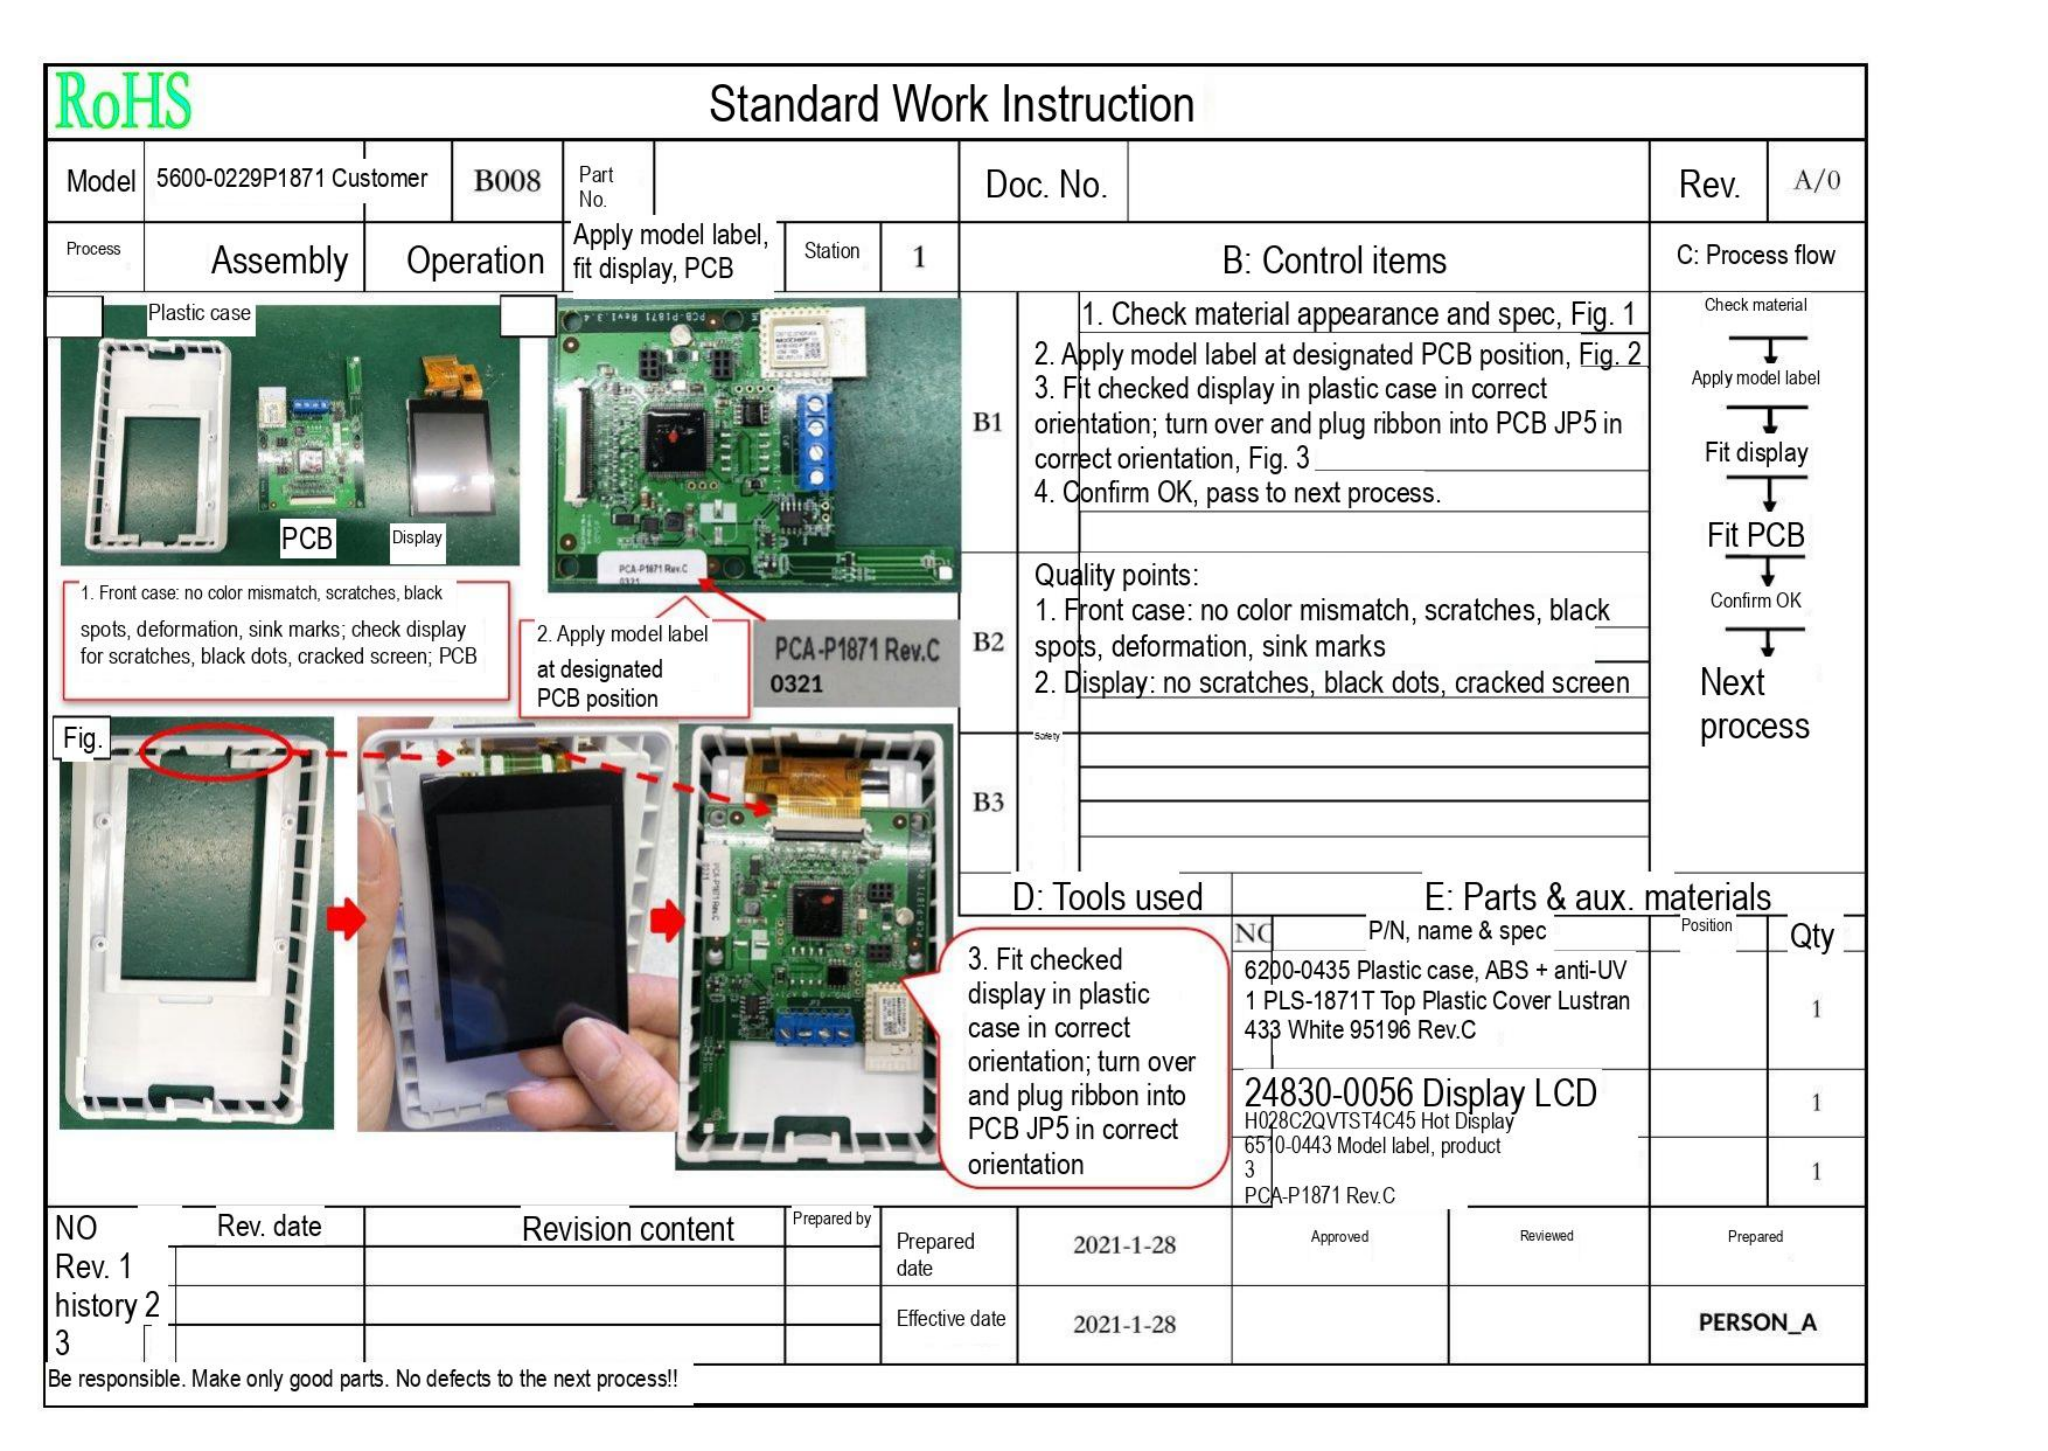RoHS

# Standard Work Instruction

| Model | 5600-0229P1871 Customer | B008 | Part No. | | Doc. No. | | Rev. | A/0 |
|---|---|---|---|---|---|---|---|---|

| Process | Assembly | Operation | Apply model label, fit display, PCB | Station | 1 | B: Control items | C: Process flow |
|---|---|---|---|---|---|---|---|

Plastic case

PCB

Display

1. Front case: no color mismatch, scratches, black spots, deformation, sink marks; check display for scratches, black dots, cracked screen; PCB

PCA-P1871 Rev.C
0321

2. Apply model label at designated PCB position

PCA-P1871 Rev.C
0321

Fig.

3. Fit checked display in plastic case in correct orientation; turn over and plug ribbon into PCB JP5 in correct orientation

| | |
|---|---|
| B1 | 1. Check material appearance and spec, Fig. 1<br>2. Apply model label at designated PCB position, Fig. 2<br>3. Fit checked display in plastic case in correct orientation; turn over and plug ribbon into PCB JP5 in correct orientation, Fig. 3<br>4. Confirm OK, pass to next process. |
| B2 | Quality points:<br>1. Front case: no color mismatch, scratches, black spots, deformation, sink marks<br>2. Display: no scratches, black dots, cracked screen |
| B3 | Safety |

C: Process flow
Check material
Apply model label
Fit display
Fit PCB
Confirm OK
Next process

D: Tools used

E: Parts & aux. materials

| NO | P/N, name & spec | Position | Qty |
|---|---|---|---|
| 1 | 6200-0435 Plastic case, ABS + anti-UV PLS-1871T Top Plastic Cover Lustran 433 White 95196 Rev.C | | 1 |
| | 24830-0056 Display LCD H028C2QVTST4C45 Hot Display | | 1 |
| 3 | 6510-0443 Model label, product PCA-P1871 Rev.C | | 1 |

| NO | Rev. date | Revision content | Prepared by |
|---|---|---|---|
| Rev. history 1 | | | |
| 2 | | | |
| 3 | | | |

| Prepared date | 2021-1-28 | Approved | Reviewed | Prepared |
|---|---|---|---|---|
| Effective date | 2021-1-28 | | | PERSON_A |

Be responsible. Make only good parts. No defects to the next process!!
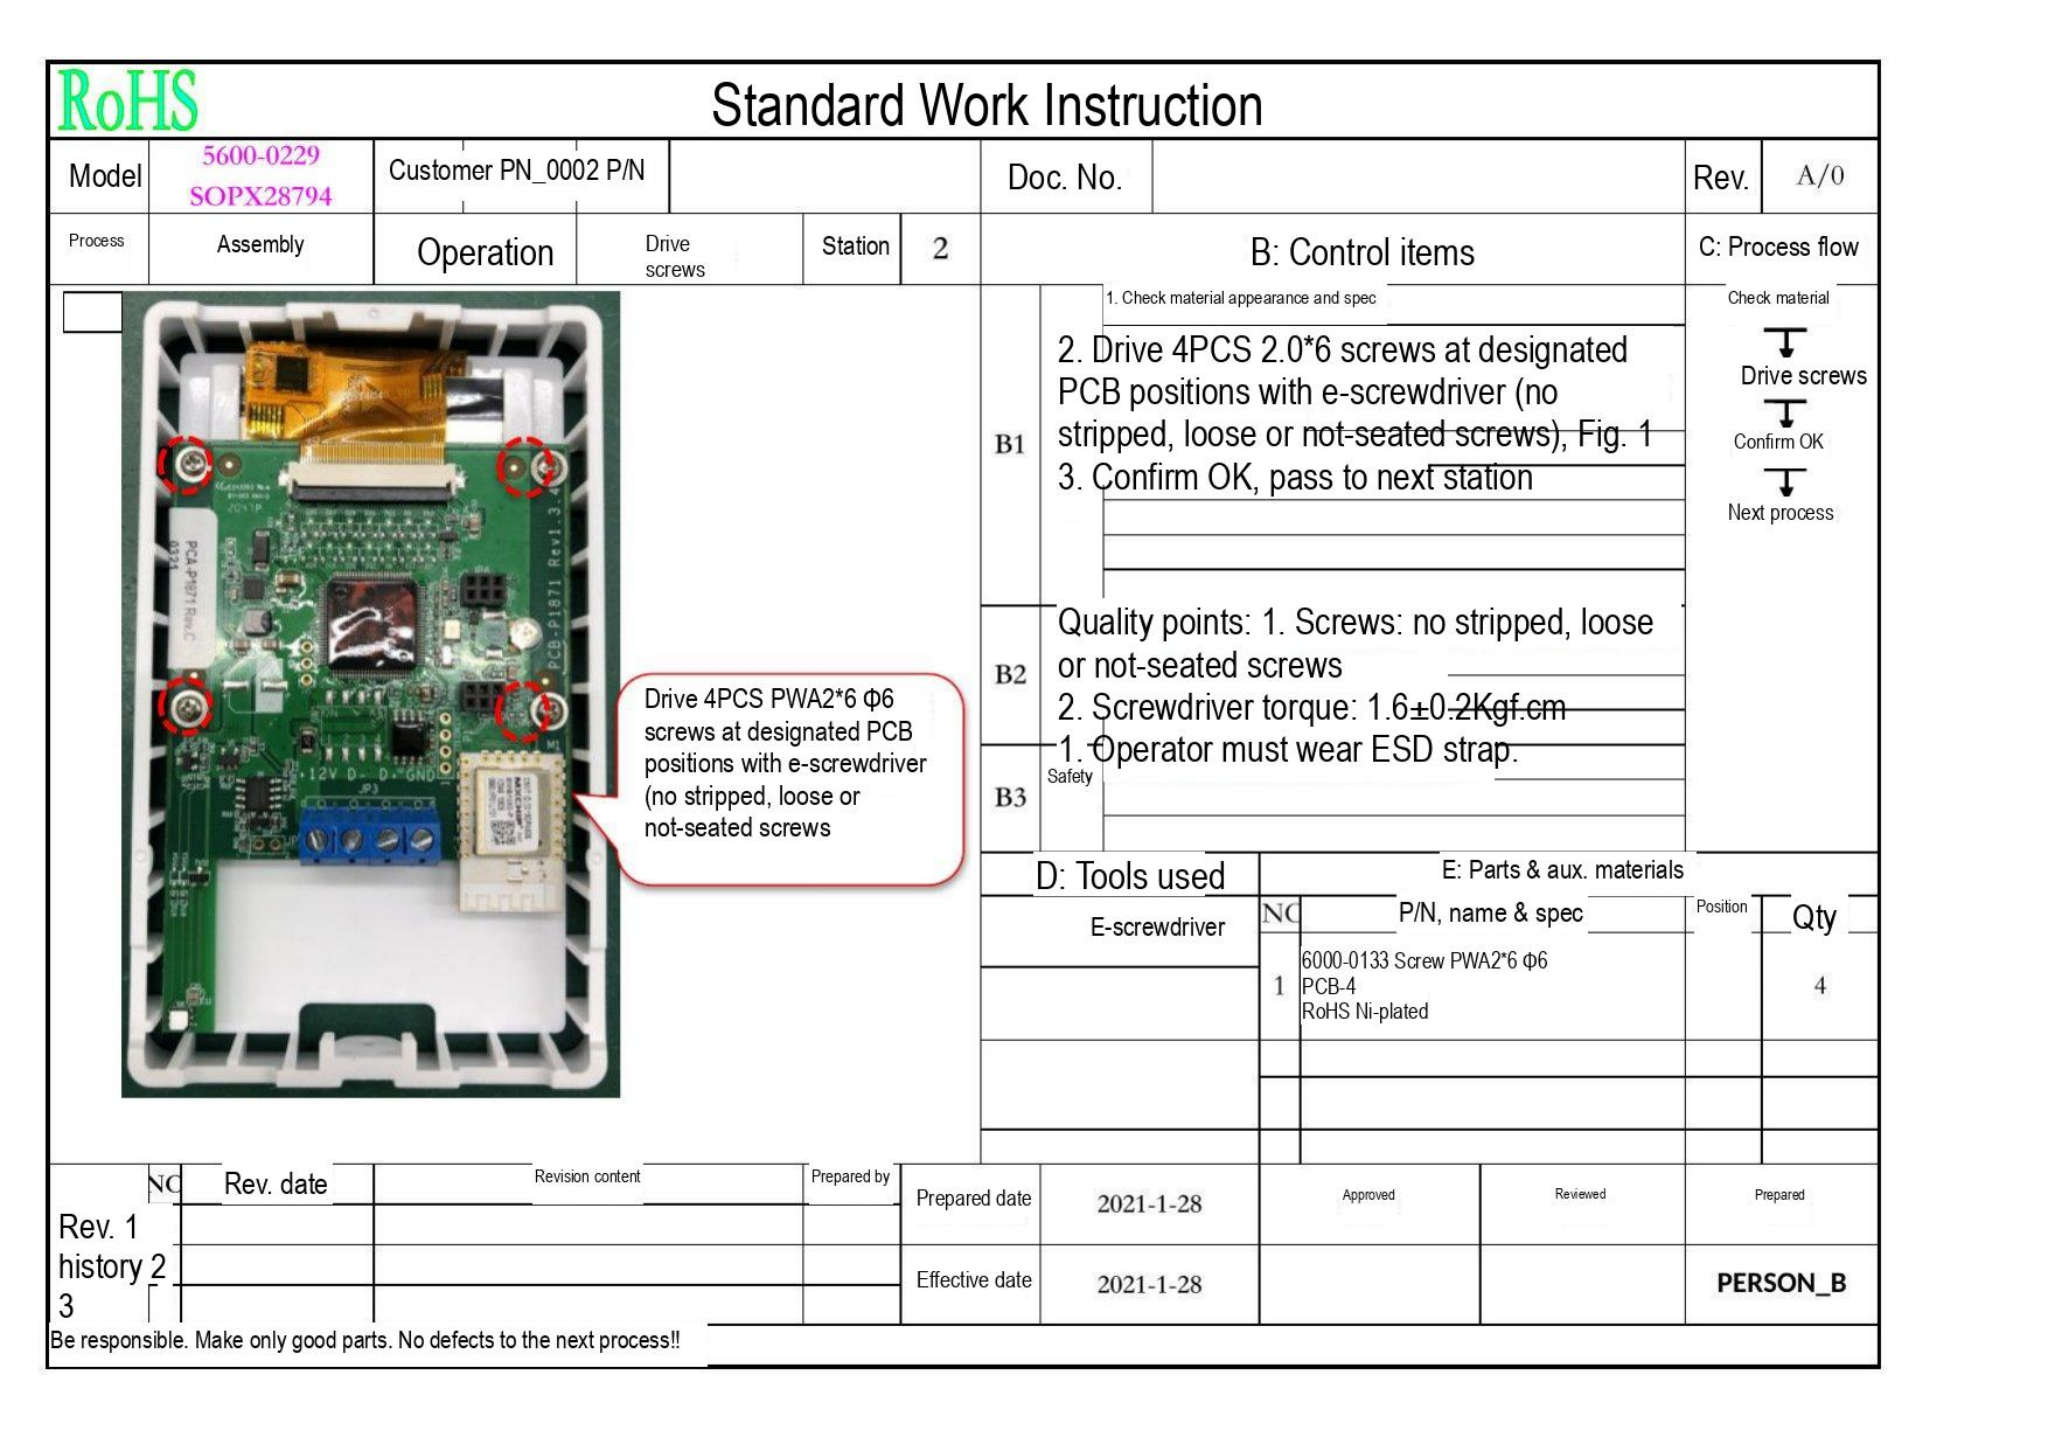RoHS

# Standard Work Instruction

| Model | 5600-0229 SOPX28794 | Customer PN_0002 P/N | | Doc. No. | | Rev. | A/0 |
|---|---|---|---|---|---|---|---|
| Process | Assembly | Operation | Drive screws | Station | 2 | | |

PCA-P1871 Rev.C

PCB-P1871 Rev1.3

12V D- D+ GND

JP3

Drive 4PCS PWA2*6 Φ6 screws at designated PCB positions with e-screwdriver (no stripped, loose or not-seated screws

**B: Control items**

| | | |
|---|---|---|
| B1 | | 1. Check material appearance and spec<br>2. Drive 4PCS 2.0*6 screws at designated PCB positions with e-screwdriver (no stripped, loose or not-seated screws), Fig. 1<br>3. Confirm OK, pass to next station |
| B2 | | Quality points: 1. Screws: no stripped, loose or not-seated screws<br>2. Screwdriver torque: 1.6±0.2Kgf.cm |
| B3 | Safety | 1. Operator must wear ESD strap. |

**C: Process flow**

Check material
↓
Drive screws
↓
Confirm OK
↓
Next process

**D: Tools used**

| D: Tools used |
|---|
| E-screwdriver |

**E: Parts & aux. materials**

| NO | P/N, name & spec | Position | Qty |
|---|---|---|---|
| 1 | 6000-0133 Screw PWA2*6 Φ6<br>PCB-4<br>RoHS Ni-plated | | 4 |

| Rev. history | NO | Rev. date | Revision content | Prepared by |
|---|---|---|---|---|
| | 1 | | | |
| | 2 | | | |
| | 3 | | | |

| Prepared date | 2021-1-28 | Approved | Reviewed | Prepared |
|---|---|---|---|---|
| Effective date | 2021-1-28 | | | PERSON_B |

Be responsible. Make only good parts. No defects to the next process!!
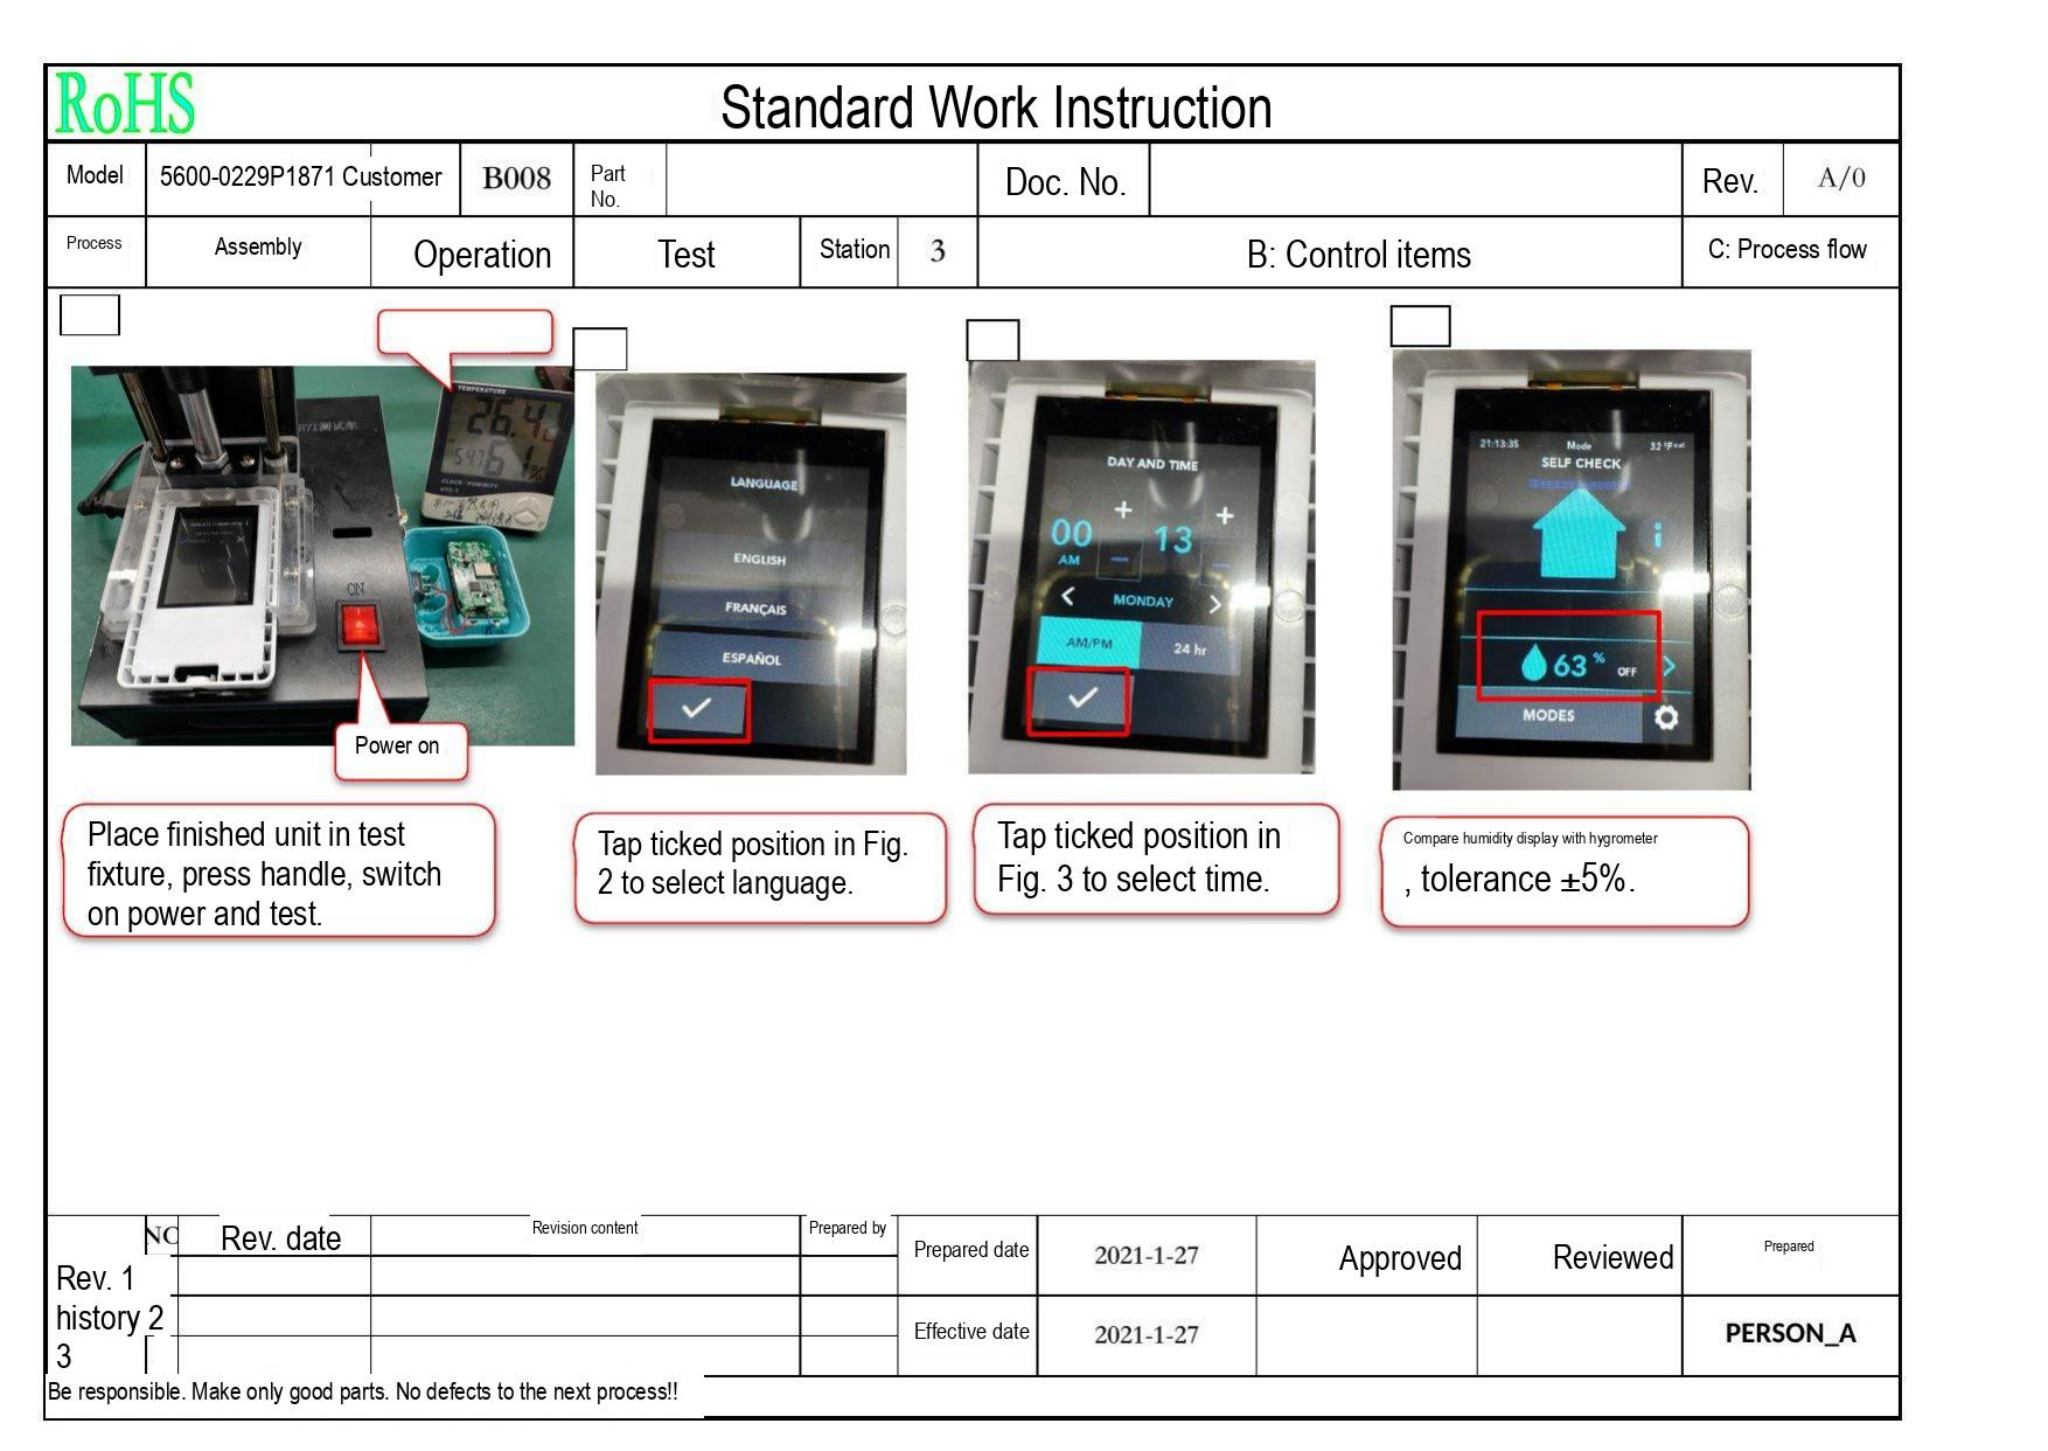RoHS

Standard Work Instruction

| Model | 5600-0229P1871 Customer | B008 | Part No. | | Doc. No. | | Rev. | A/0 |
|---|---|---|---|---|---|---|---|---|
| Process | Assembly | Operation | Test | Station | 3 | B: Control items | | C: Process flow |

TEMPERATURE
26.4
54%
61%
CLOCK HUMIDITY

ON

Power on

Place finished unit in test fixture, press handle, switch on power and test.

LANGUAGE
ENGLISH
FRANÇAIS
ESPAÑOL

Tap ticked position in Fig. 2 to select language.

DAY AND TIME
00
AM
13
MONDAY
AM/PM
24 hr

Tap ticked position in Fig. 3 to select time.

21:13:35
Mode
SELF CHECK
63 %
OFF
MODES

Compare humidity display with hygrometer
, tolerance ±5%.

| Rev. history | NO | Rev. date | Revision content | Prepared by | Prepared date | 2021-1-27 | Approved | Reviewed | Prepared |
|---|---|---|---|---|---|---|---|---|---|
| | 1 | | | | | | | | |
| | 2 | | | | Effective date | 2021-1-27 | | | PERSON_A |
| | 3 | | | | | | | | |

Be responsible. Make only good parts. No defects to the next process!!
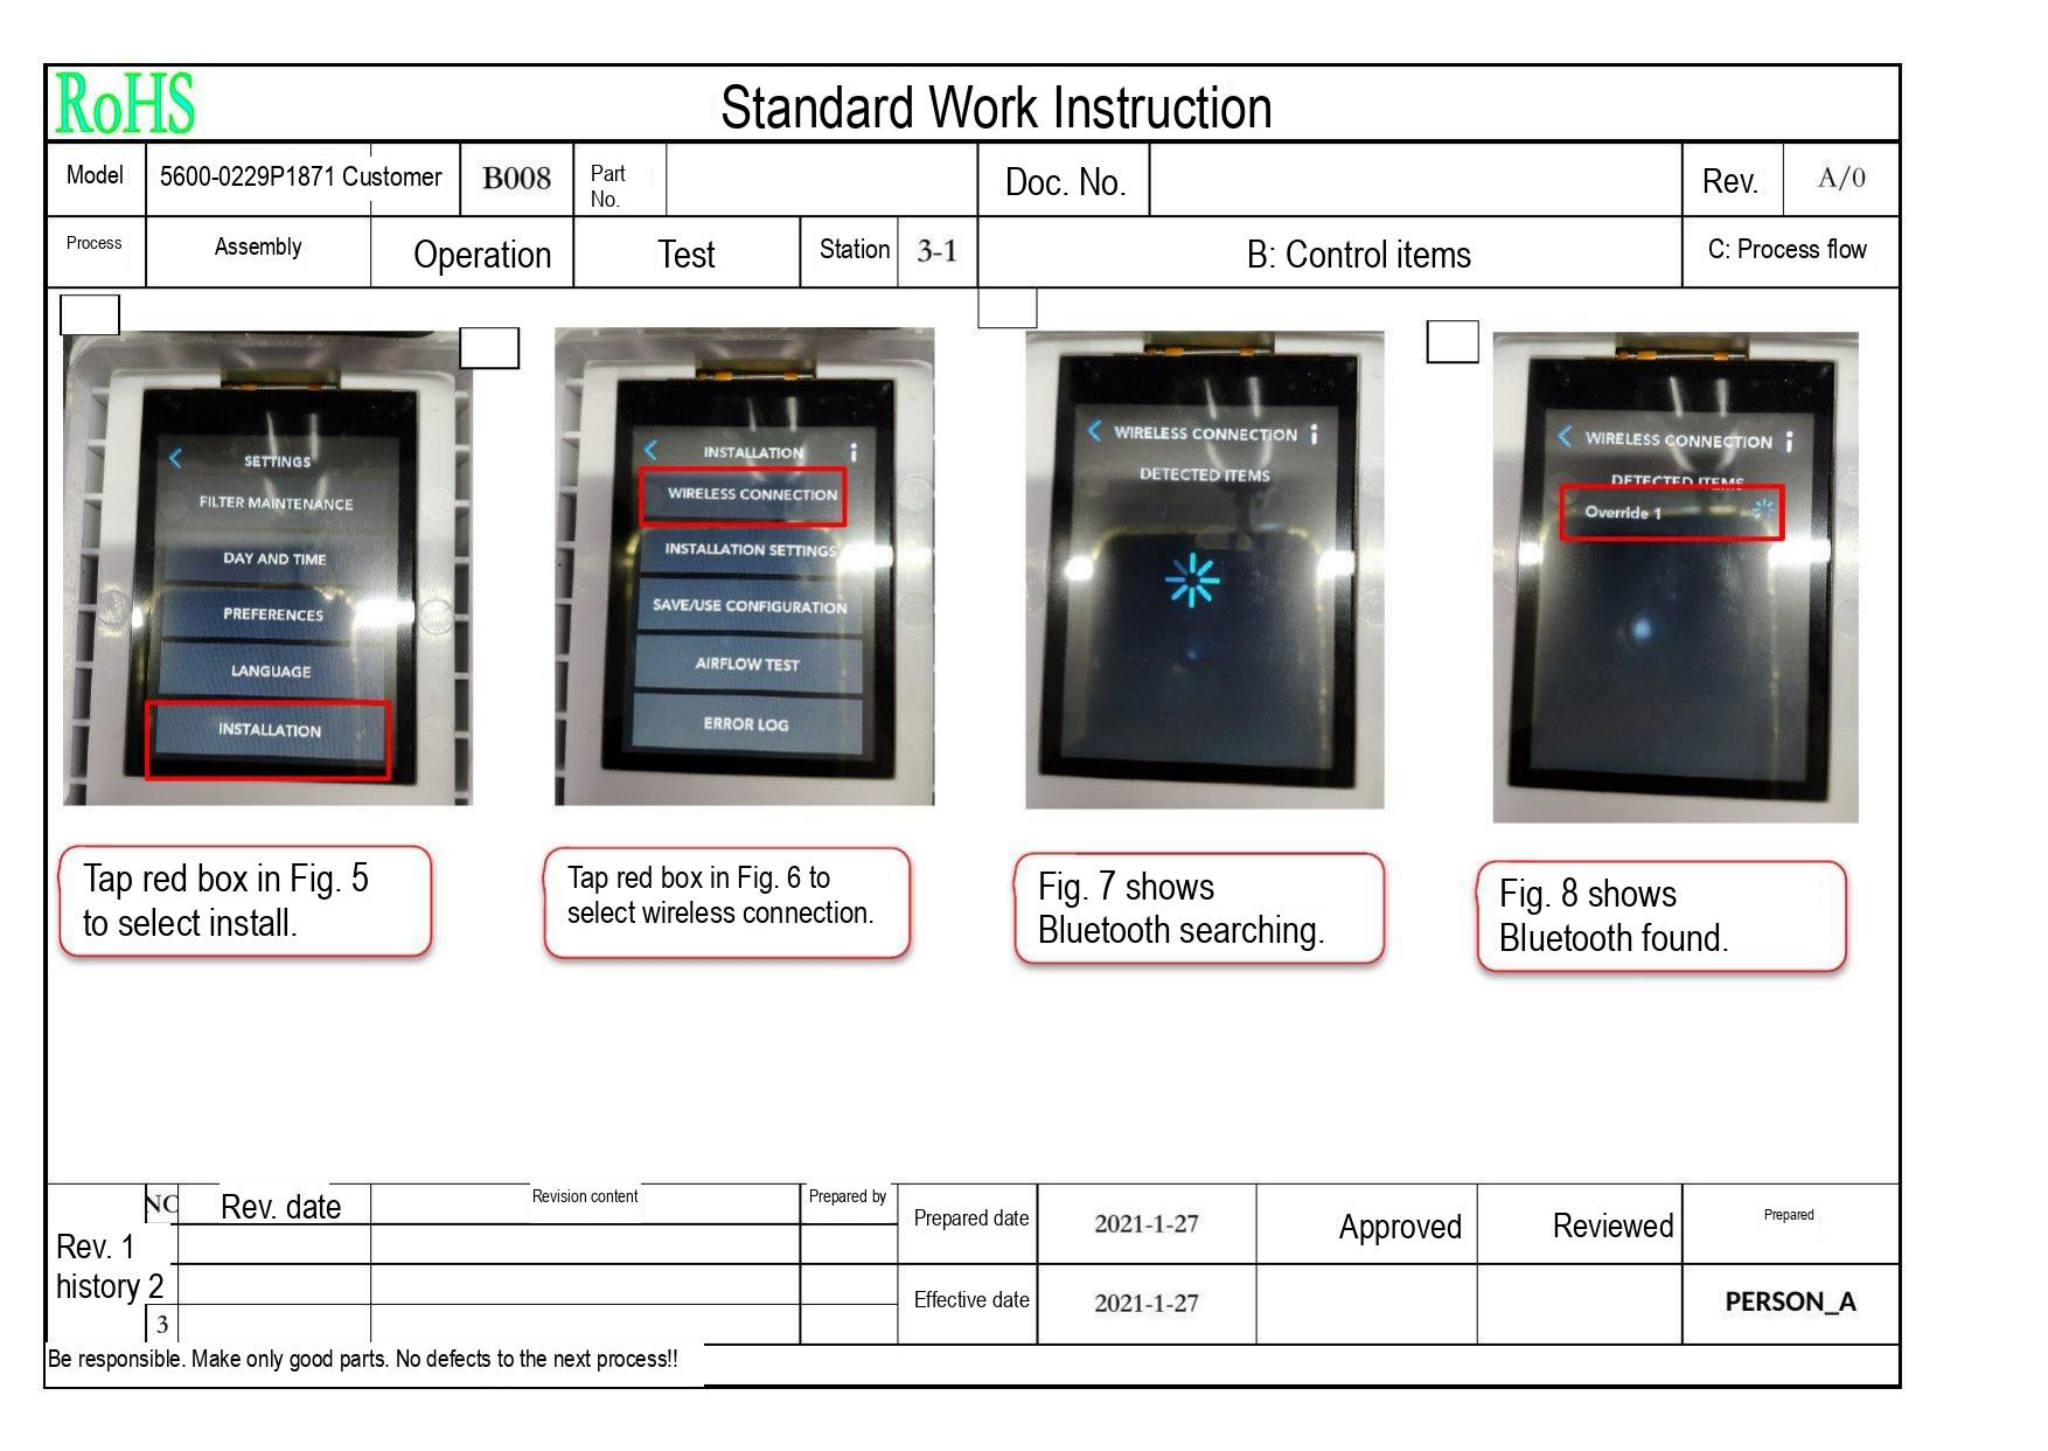RoHS

Standard Work Instruction

| Model | 5600-0229P1871 | Customer | B008 | Part No. | | Doc. No. | | Rev. | A/0 |
|---|---|---|---|---|---|---|---|---|---|
| Process | Assembly | Operation | Test | Station | 3-1 | B: Control items | | C: Process flow | |

SETTINGS
FILTER MAINTENANCE
DAY AND TIME
PREFERENCES
LANGUAGE
INSTALLATION

INSTALLATION
WIRELESS CONNECTION
INSTALLATION SETTINGS
SAVE/USE CONFIGURATION
AIRFLOW TEST
ERROR LOG

WIRELESS CONNECTION
DETECTED ITEMS

WIRELESS CONNECTION
DETECTED ITEMS
Override 1

Tap red box in Fig. 5 to select install.

Tap red box in Fig. 6 to select wireless connection.

Fig. 7 shows Bluetooth searching.

Fig. 8 shows Bluetooth found.

| Rev. history | NO | Rev. date | Revision content | Prepared by | Prepared date | 2021-1-27 | Approved | Reviewed | Prepared |
|---|---|---|---|---|---|---|---|---|---|
| | 1 | | | | | | | | |
| | 2 | | | | Effective date | 2021-1-27 | | | PERSON_A |
| | 3 | | | | | | | | |

Be responsible. Make only good parts. No defects to the next process!!
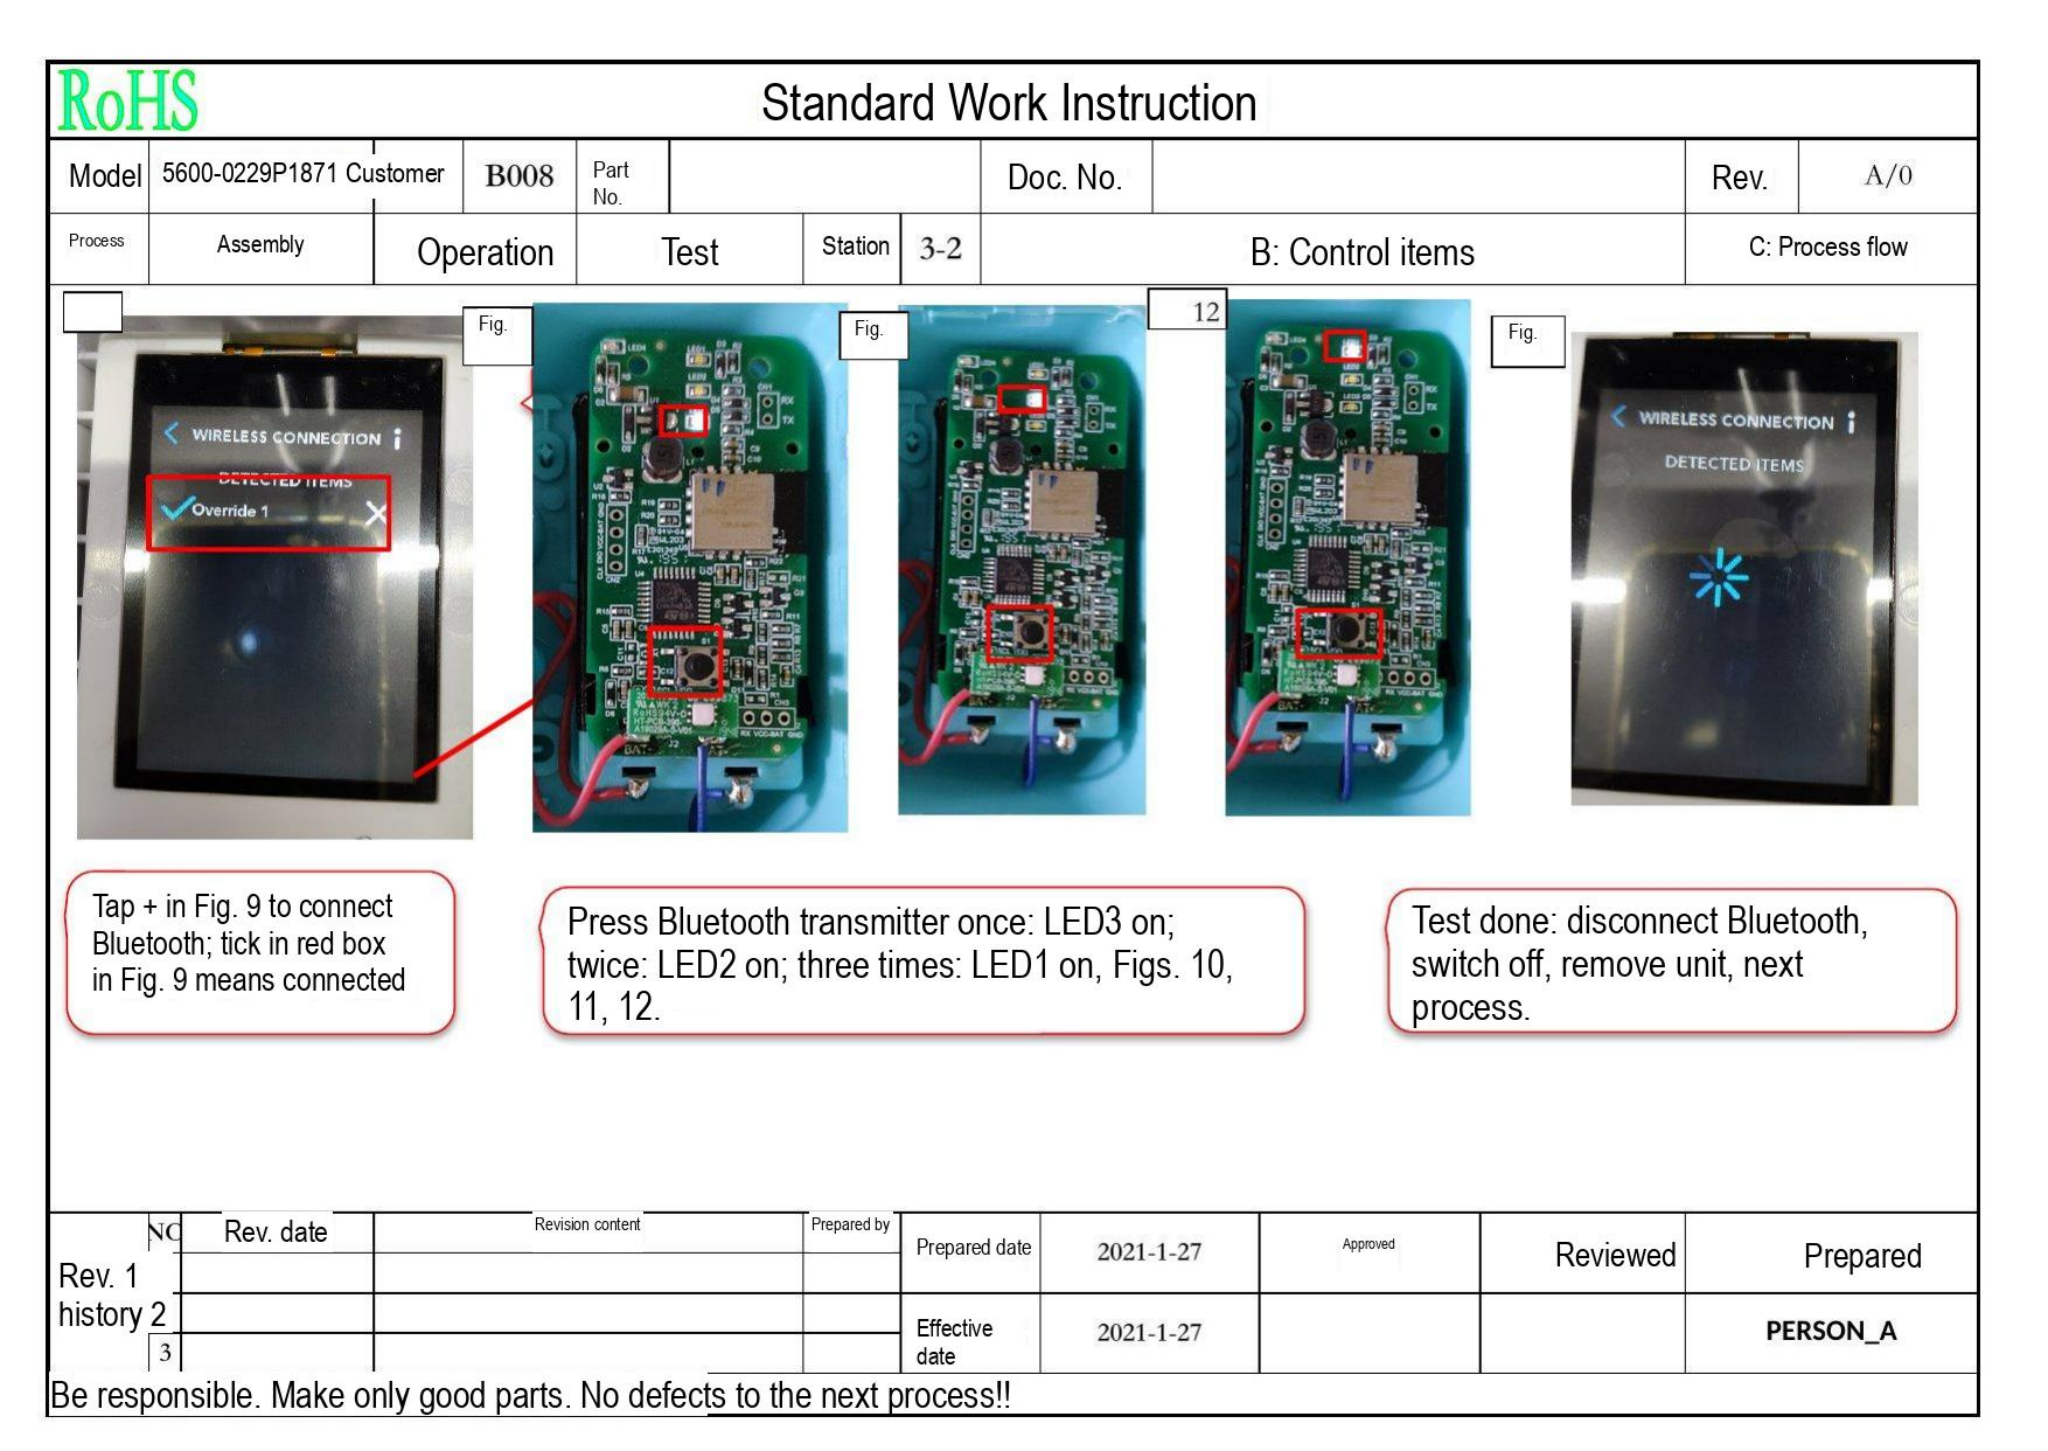RoHS

Standard Work Instruction

| Model | 5600-0229P1871 Customer | B008 | Part No. | | Doc. No. | | Rev. | A/0 |
|---|---|---|---|---|---|---|---|---|
| Process | Assembly | Operation | Test | Station | 3-2 | B: Control items | C: Process flow | |

Fig. Fig. 12 Fig.

WIRELESS CONNECTION
DETECTED ITEMS
Override 1

WIRELESS CONNECTION
DETECTED ITEMS

Tap + in Fig. 9 to connect Bluetooth; tick in red box in Fig. 9 means connected

Press Bluetooth transmitter once: LED3 on; twice: LED2 on; three times: LED1 on, Figs. 10, 11, 12.

Test done: disconnect Bluetooth, switch off, remove unit, next process.

| Rev. history | NO | Rev. date | Revision content | Prepared by | Prepared date | 2021-1-27 | Approved | Reviewed | Prepared |
|---|---|---|---|---|---|---|---|---|---|
| | 1 | | | | Effective date | 2021-1-27 | | | PERSON_A |
| | 2 | | | | | | | | |
| | 3 | | | | | | | | |

Be responsible. Make only good parts. No defects to the next process!!
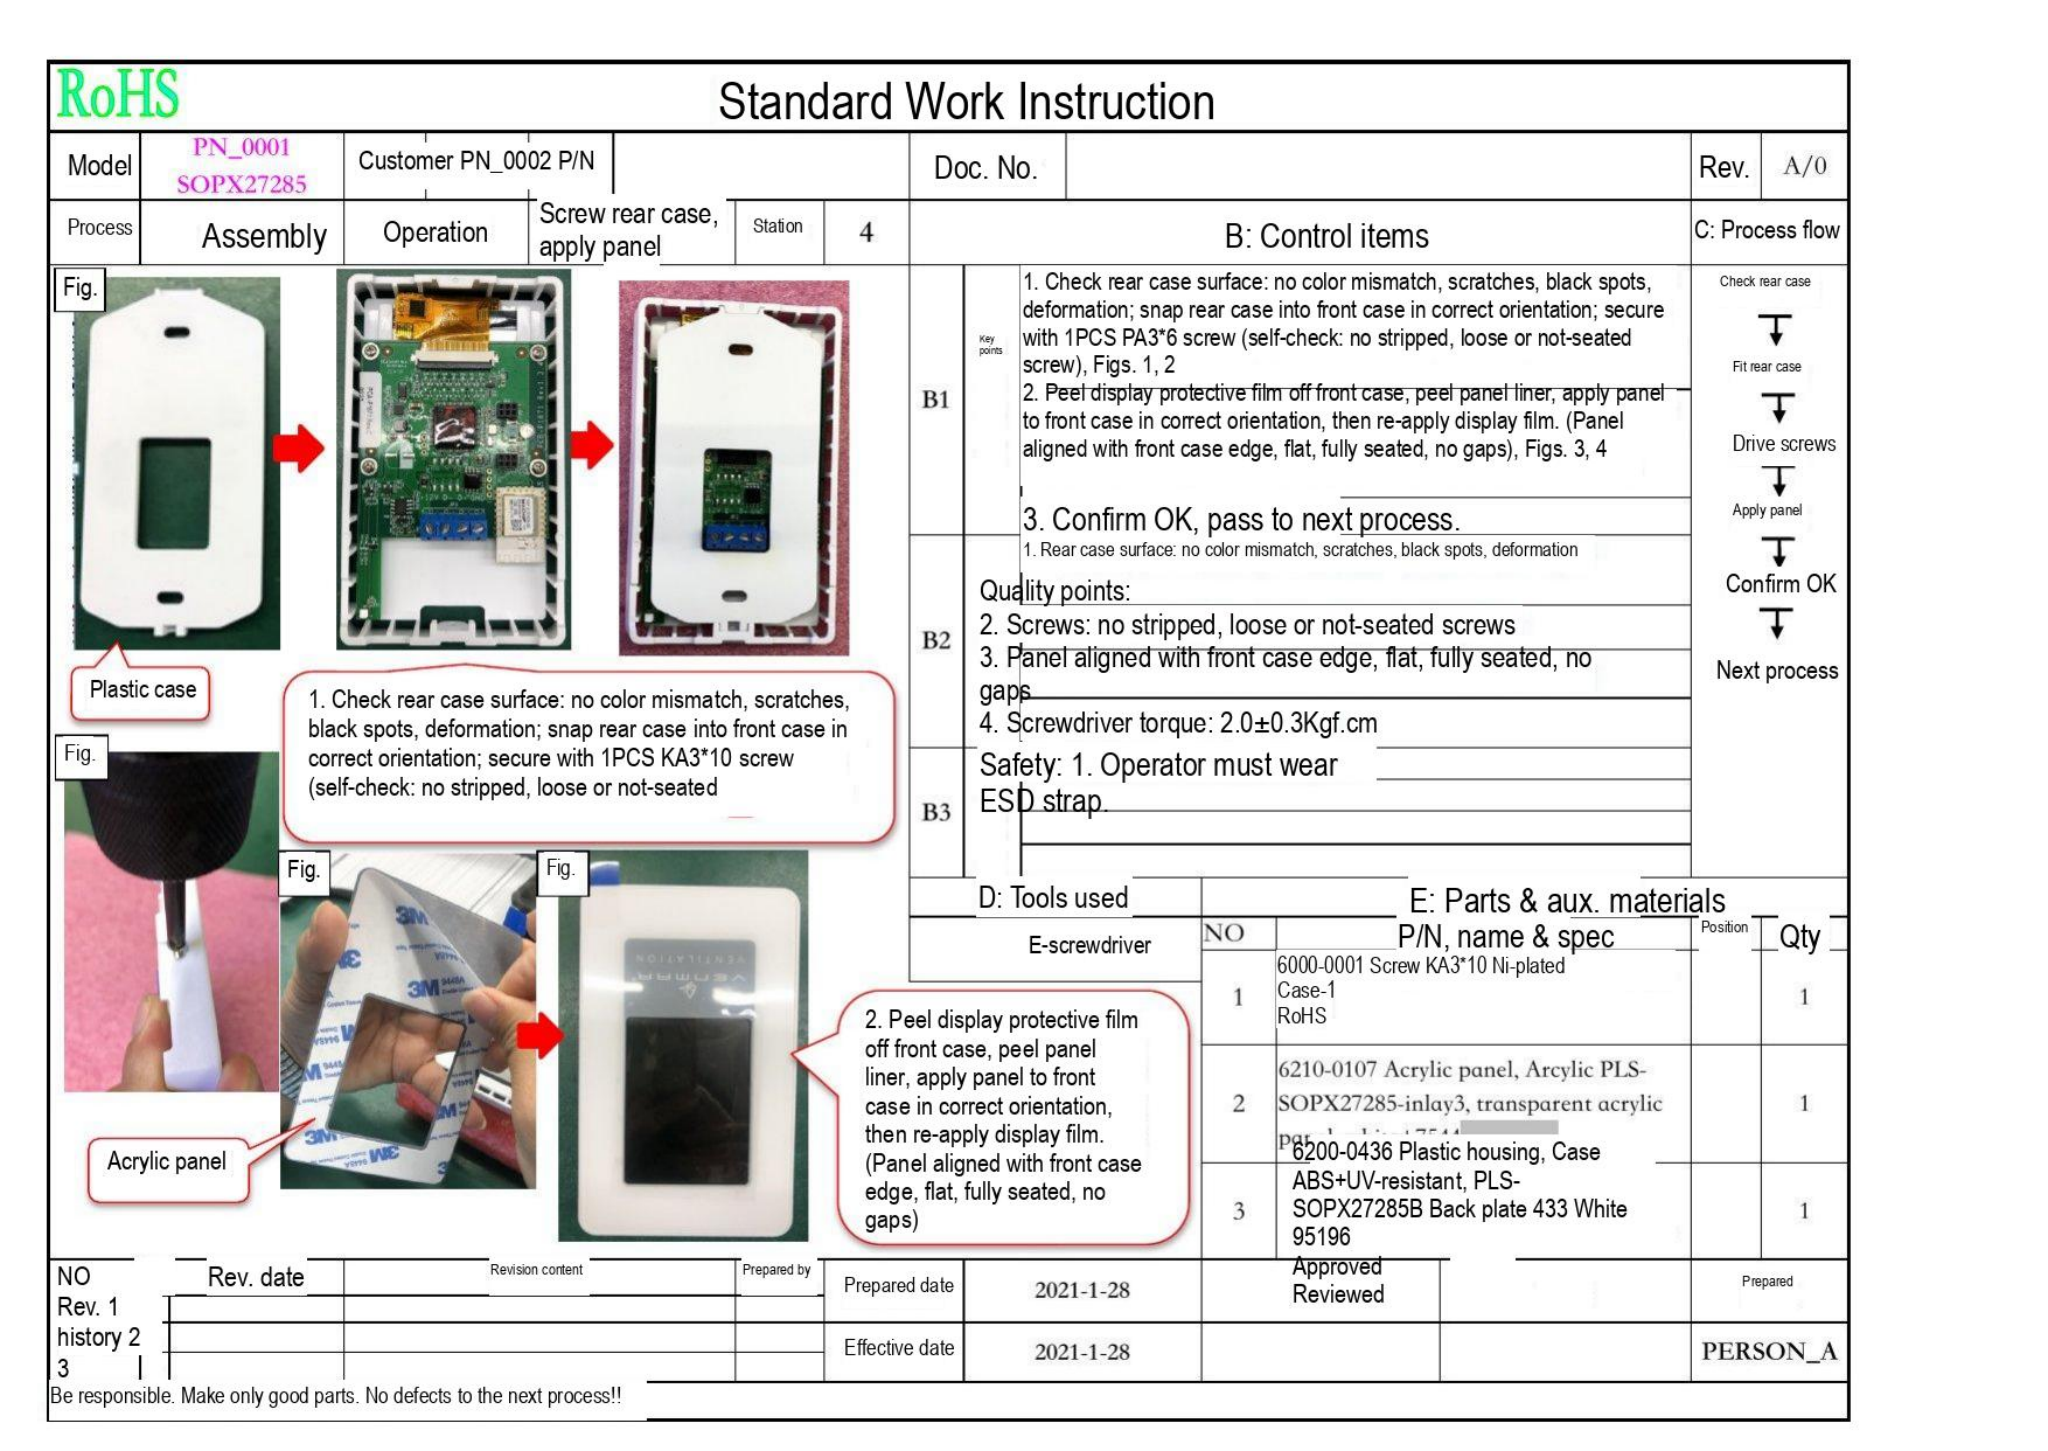RoHS

Standard Work Instruction

| Model | PN_0001 SOPX27285 | Customer PN_0002 P/N | | Doc. No. | | Rev. | A/0 |
|---|---|---|---|---|---|---|---|
| Process | Assembly | Operation | Screw rear case, apply panel | Station | 4 | B: Control items | C: Process flow |

Fig.

Fig.

Fig.

Fig.

Plastic case

1. Check rear case surface: no color mismatch, scratches, black spots, deformation; snap rear case into front case in correct orientation; secure with 1PCS KA3*10 screw (self-check: no stripped, loose or not-seated

Acrylic panel

2. Peel display protective film off front case, peel panel liner, apply panel to front case in correct orientation, then re-apply display film. (Panel aligned with front case edge, flat, fully seated, no gaps)

| | | |
|---|---|---|
| B1 | Key points | 1. Check rear case surface: no color mismatch, scratches, black spots, deformation; snap rear case into front case in correct orientation; secure with 1PCS PA3*6 screw (self-check: no stripped, loose or not-seated screw), Figs. 1, 2<br>2. Peel display protective film off front case, peel panel liner, apply panel to front case in correct orientation, then re-apply display film. (Panel aligned with front case edge, flat, fully seated, no gaps), Figs. 3, 4<br>3. Confirm OK, pass to next process. |
| B2 | | 1. Rear case surface: no color mismatch, scratches, black spots, deformation<br>Quality points:<br>2. Screws: no stripped, loose or not-seated screws<br>3. Panel aligned with front case edge, flat, fully seated, no gaps<br>4. Screwdriver torque: 2.0±0.3Kgf.cm |
| B3 | | Safety: 1. Operator must wear ESD strap. |

Check rear case
Fit rear case
Drive screws
Apply panel
Confirm OK
Next process

| D: Tools used | E: Parts & aux. materials | | | |
|---|---|---|---|---|
| | NO | P/N, name & spec | Position | Qty |
| E-screwdriver | 1 | 6000-0001 Screw KA3*10 Ni-plated Case-1 RoHS | | 1 |
| | 2 | 6210-0107 Acrylic panel, Arcylic PLS-SOPX27285-inlay3, transparent acrylic | | 1 |
| | 3 | 6200-0436 Plastic housing, Case ABS+UV-resistant, PLS-SOPX27285B Back plate 433 White 95196 | | 1 |

| NO | Rev. date | Revision content | Prepared by | Prepared date | 2021-1-28 | Approved Reviewed | | Prepared |
|---|---|---|---|---|---|---|---|---|
| Rev. 1 | | | | | | | | |
| history 2 | | | | Effective date | 2021-1-28 | | | PERSON_A |
| 3 | | | | | | | | |

Be responsible. Make only good parts. No defects to the next process!!